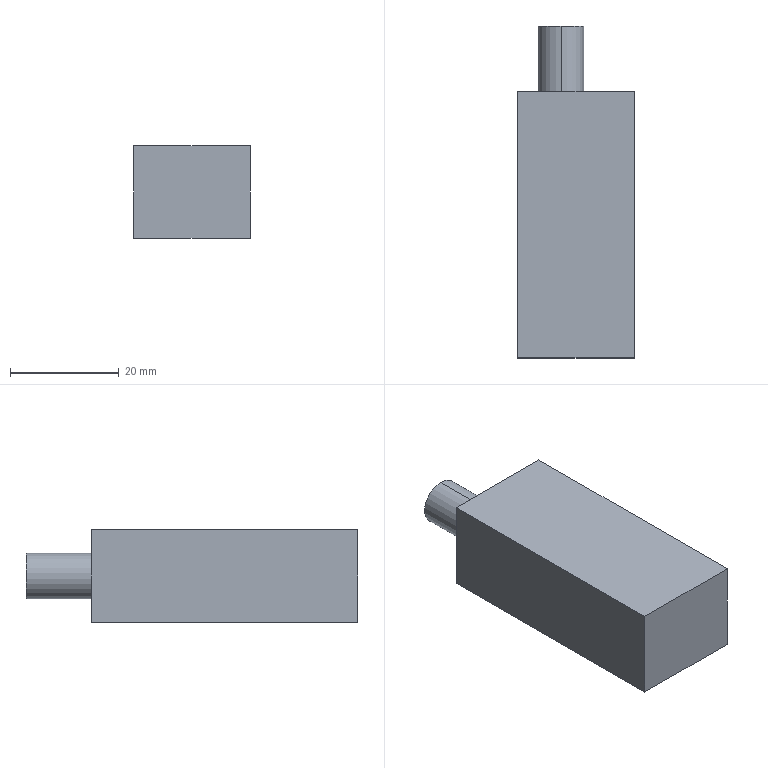Part | CATIA | 1 solid | 9 faces | box 21.5 x 61 x 17 mm | volume 18577 mm3 | plane 7 | cylinder 2 | commonest cylinder face diameters 8.413 x2
STEP:
#1=CARTESIAN_POINT('',(13.5,37.2,12.706));
#2=VERTEX_POINT('',#1);
#3=CARTESIAN_POINT('',(13.5,49.2,12.706));
#4=VERTEX_POINT('',#3);
#5=CARTESIAN_POINT('',(13.5,43.2,12.706));
#6=DIRECTION('',(0.,1.,0.));
#7=VECTOR('',#6,1.);
#8=LINE('',#5,#7);
#9=EDGE_CURVE('',#2,#4,#8,.T.);
#10=ORIENTED_EDGE('',*,*,#9,.F.);
#11=CARTESIAN_POINT('',(13.5,37.2,4.294));
#12=VERTEX_POINT('',#11);
#13=CARTESIAN_POINT('',(13.5,37.2,8.5));
#14=DIRECTION('',(0.,1.,0.));
#15=AXIS2_PLACEMENT_3D('',#13,#14,$);
#16=CIRCLE('',#15,4.206);
#17=EDGE_CURVE('',#2,#12,#16,.T.);
#18=ORIENTED_EDGE('',*,*,#17,.T.);
#19=CARTESIAN_POINT('',(13.5,49.2,4.294));
#20=VERTEX_POINT('',#19);
#21=CARTESIAN_POINT('',(13.5,43.2,4.294));
#22=DIRECTION('',(0.,1.,0.));
#23=VECTOR('',#22,1.);
#24=LINE('',#21,#23);
#25=EDGE_CURVE('',#12,#20,#24,.T.);
#26=ORIENTED_EDGE('',*,*,#25,.T.);
#27=CARTESIAN_POINT('',(13.5,49.2,8.5));
#28=DIRECTION('',(0.,1.,0.));
#29=AXIS2_PLACEMENT_3D('',#27,#28,$);
#30=CIRCLE('',#29,4.206);
#31=EDGE_CURVE('',#4,#20,#30,.T.);
#32=ORIENTED_EDGE('',*,*,#31,.F.);
#33=EDGE_LOOP('',(#10,#18,#26,#32));
#34=FACE_OUTER_BOUND('',#33,.T.);
#35=CARTESIAN_POINT('',(13.5,43.2,8.5));
#36=DIRECTION('',(0.,1.,0.));
#37=DIRECTION('',(0.,0.,1.));
#38=AXIS2_PLACEMENT_3D('',#35,#36,#37);
#39=CYLINDRICAL_SURFACE('',#38,4.206);
#40=ADVANCED_FACE('',(#34),#39,.T.);
#41=ORIENTED_EDGE('',*,*,#25,.F.);
#42=CARTESIAN_POINT('',(13.5,37.2,8.5));
#43=DIRECTION('',(0.,1.,0.));
#44=AXIS2_PLACEMENT_3D('',#42,#43,$);
#45=CIRCLE('',#44,4.206);
#46=EDGE_CURVE('',#12,#2,#45,.T.);
#47=ORIENTED_EDGE('',*,*,#46,.T.);
#48=ORIENTED_EDGE('',*,*,#9,.T.);
#49=CARTESIAN_POINT('',(13.5,49.2,8.5));
#50=DIRECTION('',(0.,1.,0.));
#51=AXIS2_PLACEMENT_3D('',#49,#50,$);
#52=CIRCLE('',#51,4.206);
#53=EDGE_CURVE('',#20,#4,#52,.T.);
#54=ORIENTED_EDGE('',*,*,#53,.F.);
#55=EDGE_LOOP('',(#41,#47,#48,#54));
#56=FACE_OUTER_BOUND('',#55,.T.);
#57=CARTESIAN_POINT('',(13.5,43.2,8.5));
#58=DIRECTION('',(0.,1.,0.));
#59=DIRECTION('',(0.,0.,-1.));
#60=AXIS2_PLACEMENT_3D('',#57,#58,#59);
#61=CYLINDRICAL_SURFACE('',#60,4.206);
#62=ADVANCED_FACE('',(#56),#61,.T.);
#63=CARTESIAN_POINT('',(27.,37.2,0.));
#64=VERTEX_POINT('',#63);
#65=CARTESIAN_POINT('',(27.,37.2,17.));
#66=VERTEX_POINT('',#65);
#67=CARTESIAN_POINT('',(27.,37.2,8.5));
#68=DIRECTION('',(0.,0.,1.));
#69=VECTOR('',#68,1.);
#70=LINE('',#67,#69);
#71=EDGE_CURVE('',#64,#66,#70,.T.);
#72=ORIENTED_EDGE('',*,*,#71,.F.);
#73=CARTESIAN_POINT('',(5.5,37.2,0.));
#74=VERTEX_POINT('',#73);
#75=CARTESIAN_POINT('',(16.25,37.2,0.));
#76=DIRECTION('',(1.,0.,0.));
#77=VECTOR('',#76,1.);
#78=LINE('',#75,#77);
#79=EDGE_CURVE('',#64,#74,#78,.F.);
#80=ORIENTED_EDGE('',*,*,#79,.T.);
#81=CARTESIAN_POINT('',(5.5,37.2,17.));
#82=VERTEX_POINT('',#81);
#83=CARTESIAN_POINT('',(5.5,37.2,8.5));
#84=DIRECTION('',(0.,0.,1.));
#85=VECTOR('',#84,1.);
#86=LINE('',#83,#85);
#87=EDGE_CURVE('',#74,#82,#86,.T.);
#88=ORIENTED_EDGE('',*,*,#87,.T.);
#89=CARTESIAN_POINT('',(16.25,37.2,17.));
#90=DIRECTION('',(1.,0.,0.));
#91=VECTOR('',#90,1.);
#92=LINE('',#89,#91);
#93=EDGE_CURVE('',#66,#82,#92,.F.);
#94=ORIENTED_EDGE('',*,*,#93,.F.);
#95=EDGE_LOOP('',(#72,#80,#88,#94));
#96=FACE_OUTER_BOUND('',#95,.T.);
#97=ORIENTED_EDGE('',*,*,#46,.F.);
#98=ORIENTED_EDGE('',*,*,#17,.F.);
#99=EDGE_LOOP('',(#97,#98));
#100=FACE_BOUND('',#99,.T.);
#101=CARTESIAN_POINT('',(5.5,37.2,0.));
#102=DIRECTION('',(0.,-1.,0.));
#103=DIRECTION('',(1.,0.,0.));
#104=AXIS2_PLACEMENT_3D('',#101,#102,#103);
#105=PLANE('',#104);
#106=ADVANCED_FACE('',(#96,#100),#105,.F.);
#107=ORIENTED_EDGE('',*,*,#31,.T.);
#108=ORIENTED_EDGE('',*,*,#53,.T.);
#109=EDGE_LOOP('',(#107,#108));
#110=FACE_OUTER_BOUND('',#109,.T.);
#111=CARTESIAN_POINT('',(0.,49.2,0.));
#112=DIRECTION('',(0.,1.,0.));
#113=DIRECTION('',(-1.,0.,0.));
#114=AXIS2_PLACEMENT_3D('',#111,#112,#113);
#115=PLANE('',#114);
#116=ADVANCED_FACE('',(#110),#115,.T.);
#117=CARTESIAN_POINT('',(27.,-11.8,0.));
#118=VERTEX_POINT('',#117);
#119=CARTESIAN_POINT('',(27.,-11.8,17.));
#120=VERTEX_POINT('',#119);
#121=CARTESIAN_POINT('',(27.,-11.8,8.5));
#122=DIRECTION('',(0.,0.,1.));
#123=VECTOR('',#122,1.);
#124=LINE('',#121,#123);
#125=EDGE_CURVE('',#118,#120,#124,.T.);
#126=ORIENTED_EDGE('',*,*,#125,.F.);
#127=CARTESIAN_POINT('',(27.,12.7,0.));
#128=DIRECTION('',(0.,1.,0.));
#129=VECTOR('',#128,1.);
#130=LINE('',#127,#129);
#131=EDGE_CURVE('',#118,#64,#130,.T.);
#132=ORIENTED_EDGE('',*,*,#131,.T.);
#133=ORIENTED_EDGE('',*,*,#71,.T.);
#134=CARTESIAN_POINT('',(27.,12.7,17.));
#135=DIRECTION('',(0.,1.,0.));
#136=VECTOR('',#135,1.);
#137=LINE('',#134,#136);
#138=EDGE_CURVE('',#120,#66,#137,.T.);
#139=ORIENTED_EDGE('',*,*,#138,.F.);
#140=EDGE_LOOP('',(#126,#132,#133,#139));
#141=FACE_OUTER_BOUND('',#140,.T.);
#142=CARTESIAN_POINT('',(27.,-11.8,0.));
#143=DIRECTION('',(1.,0.,0.));
#144=DIRECTION('',(0.,1.,0.));
#145=AXIS2_PLACEMENT_3D('',#142,#143,#144);
#146=PLANE('',#145);
#147=ADVANCED_FACE('',(#141),#146,.T.);
#148=ORIENTED_EDGE('',*,*,#79,.F.);
#149=ORIENTED_EDGE('',*,*,#131,.F.);
#150=CARTESIAN_POINT('',(5.5,-11.8,0.));
#151=VERTEX_POINT('',#150);
#152=CARTESIAN_POINT('',(16.25,-11.8,0.));
#153=DIRECTION('',(-1.,0.,0.));
#154=VECTOR('',#153,1.);
#155=LINE('',#152,#154);
#156=EDGE_CURVE('',#151,#118,#155,.F.);
#157=ORIENTED_EDGE('',*,*,#156,.F.);
#158=CARTESIAN_POINT('',(5.5,12.7,0.));
#159=DIRECTION('',(0.,-1.,0.));
#160=VECTOR('',#159,1.);
#161=LINE('',#158,#160);
#162=EDGE_CURVE('',#74,#151,#161,.T.);
#163=ORIENTED_EDGE('',*,*,#162,.F.);
#164=EDGE_LOOP('',(#148,#149,#157,#163));
#165=FACE_OUTER_BOUND('',#164,.T.);
#166=CARTESIAN_POINT('',(0.,0.,0.));
#167=DIRECTION('',(0.,0.,1.));
#168=DIRECTION('',(1.,0.,0.));
#169=AXIS2_PLACEMENT_3D('',#166,#167,#168);
#170=PLANE('',#169);
#171=ADVANCED_FACE('',(#165),#170,.F.);
#172=ORIENTED_EDGE('',*,*,#87,.F.);
#173=ORIENTED_EDGE('',*,*,#162,.T.);
#174=CARTESIAN_POINT('',(5.5,-11.8,17.));
#175=VERTEX_POINT('',#174);
#176=CARTESIAN_POINT('',(5.5,-11.8,8.5));
#177=DIRECTION('',(0.,0.,1.));
#178=VECTOR('',#177,1.);
#179=LINE('',#176,#178);
#180=EDGE_CURVE('',#151,#175,#179,.T.);
#181=ORIENTED_EDGE('',*,*,#180,.T.);
#182=CARTESIAN_POINT('',(5.5,12.7,17.));
#183=DIRECTION('',(0.,-1.,0.));
#184=VECTOR('',#183,1.);
#185=LINE('',#182,#184);
#186=EDGE_CURVE('',#82,#175,#185,.T.);
#187=ORIENTED_EDGE('',*,*,#186,.F.);
#188=EDGE_LOOP('',(#172,#173,#181,#187));
#189=FACE_OUTER_BOUND('',#188,.T.);
#190=CARTESIAN_POINT('',(5.5,37.2,0.));
#191=DIRECTION('',(-1.,0.,0.));
#192=DIRECTION('',(0.,-1.,0.));
#193=AXIS2_PLACEMENT_3D('',#190,#191,#192);
#194=PLANE('',#193);
#195=ADVANCED_FACE('',(#189),#194,.T.);
#196=ORIENTED_EDGE('',*,*,#186,.T.);
#197=CARTESIAN_POINT('',(16.25,-11.8,17.));
#198=DIRECTION('',(-1.,0.,0.));
#199=VECTOR('',#198,1.);
#200=LINE('',#197,#199);
#201=EDGE_CURVE('',#175,#120,#200,.F.);
#202=ORIENTED_EDGE('',*,*,#201,.T.);
#203=ORIENTED_EDGE('',*,*,#138,.T.);
#204=ORIENTED_EDGE('',*,*,#93,.T.);
#205=EDGE_LOOP('',(#196,#202,#203,#204));
#206=FACE_OUTER_BOUND('',#205,.T.);
#207=CARTESIAN_POINT('',(0.,0.,17.));
#208=DIRECTION('',(0.,0.,1.));
#209=DIRECTION('',(1.,0.,0.));
#210=AXIS2_PLACEMENT_3D('',#207,#208,#209);
#211=PLANE('',#210);
#212=ADVANCED_FACE('',(#206),#211,.T.);
#213=ORIENTED_EDGE('',*,*,#180,.F.);
#214=ORIENTED_EDGE('',*,*,#156,.T.);
#215=ORIENTED_EDGE('',*,*,#125,.T.);
#216=ORIENTED_EDGE('',*,*,#201,.F.);
#217=EDGE_LOOP('',(#213,#214,#215,#216));
#218=FACE_OUTER_BOUND('',#217,.T.);
#219=CARTESIAN_POINT('',(27.,-11.8,0.));
#220=DIRECTION('',(0.,1.,0.));
#221=DIRECTION('',(-1.,0.,0.));
#222=AXIS2_PLACEMENT_3D('',#219,#220,#221);
#223=PLANE('',#222);
#224=ADVANCED_FACE('',(#218),#223,.F.);
#225=CLOSED_SHELL('',(#40,#62,#106,#116,#147,#171,#195,#212,#224));
#226=MANIFOLD_SOLID_BREP('',#225);
#227=(LENGTH_UNIT()NAMED_UNIT(*)SI_UNIT(.MILLI.,.METRE.));
#228=UNCERTAINTY_MEASURE_WITH_UNIT(LENGTH_MEASURE(0.005),#227,'','');
#229=(NAMED_UNIT(*)PLANE_ANGLE_UNIT()SI_UNIT($,.RADIAN.));
#230=(NAMED_UNIT(*)SI_UNIT($,.STERADIAN.)SOLID_ANGLE_UNIT());
#231=(GEOMETRIC_REPRESENTATION_CONTEXT(3)GLOBAL_UNCERTAINTY_ASSIGNED_CONTEXT((#228))GLOBAL_UNIT_ASSIGNED_CONTEXT((#227,#229,#230))REPRESENTATION_CONTEXT('',''));
#232=ADVANCED_BREP_SHAPE_REPRESENTATION('',(#226),#231);